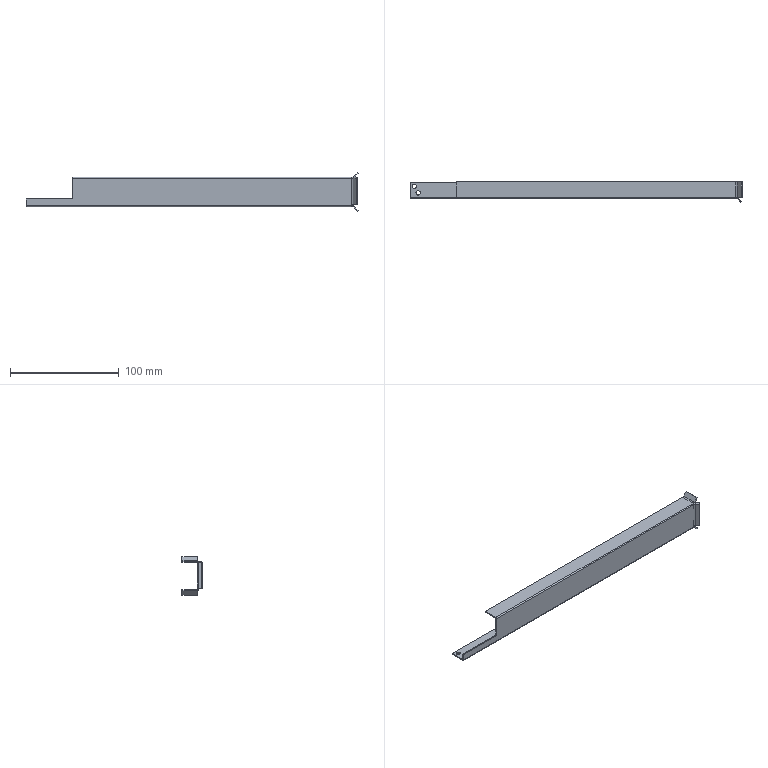Part | NX | 1 solid | 39 faces | box 305.707 x 18.464 x 35.21 mm | volume 15234 mm3 | plane 24 | cylinder 14 | torus 1 | commonest cylinder face diameters 4 x6 6 x4 2 x3 2.56 x1
STEP:
#1=CARTESIAN_POINT('',(150.133,7.5,151.5));
#2=VERTEX_POINT('',#1);
#3=CARTESIAN_POINT('',(150.133,-6.501,151.5));
#4=VERTEX_POINT('',#3);
#5=CARTESIAN_POINT('',(150.133,7.5,151.5));
#6=DIRECTION('',(0.,-1.,0.));
#7=VECTOR('',#6,1000.);
#8=LINE('',#5,#7);
#9=EDGE_CURVE('',#2,#4,#8,.T.);
#10=ORIENTED_EDGE('',*,*,#9,.F.);
#11=CARTESIAN_POINT('',(-107.,7.5,151.5));
#12=VERTEX_POINT('',#11);
#13=CARTESIAN_POINT('',(-107.,7.5,151.5));
#14=DIRECTION('',(1.,0.,0.));
#15=VECTOR('',#14,1000.);
#16=LINE('',#13,#15);
#17=EDGE_CURVE('',#12,#2,#16,.T.);
#18=ORIENTED_EDGE('',*,*,#17,.F.);
#19=CARTESIAN_POINT('',(-107.,-6.5,151.5));
#20=VERTEX_POINT('',#19);
#21=CARTESIAN_POINT('',(-107.,7.5,151.5));
#22=DIRECTION('',(0.,-1.,0.));
#23=VECTOR('',#22,1000.);
#24=LINE('',#21,#23);
#25=EDGE_CURVE('',#12,#20,#24,.T.);
#26=ORIENTED_EDGE('',*,*,#25,.T.);
#27=CARTESIAN_POINT('',(150.,-6.5,151.5));
#28=VERTEX_POINT('',#27);
#29=CARTESIAN_POINT('',(150.722,-6.5,151.5));
#30=DIRECTION('',(1.,0.,0.));
#31=VECTOR('',#30,1000.);
#32=LINE('',#29,#31);
#33=EDGE_CURVE('',#20,#28,#32,.T.);
#34=ORIENTED_EDGE('',*,*,#33,.T.);
#35=CARTESIAN_POINT('',(150.,-9.5,151.5));
#36=DIRECTION('',(0.,0.,1.));
#37=DIRECTION('',(0.04435,0.999,0.));
#38=AXIS2_PLACEMENT_3D('',#35,#36,#37);
#39=CIRCLE('',#38,3.);
#40=EDGE_CURVE('',#4,#28,#39,.T.);
#41=ORIENTED_EDGE('',*,*,#40,.F.);
#42=EDGE_LOOP('',(#10,#18,#26,#34,#41));
#43=FACE_BOUND('',#42,.T.);
#44=CARTESIAN_POINT('',(0.,0.,151.5));
#45=DIRECTION('',(0.,0.,1.));
#46=DIRECTION('',(1.,0.,0.));
#47=AXIS2_PLACEMENT_3D('',#44,#45,#46);
#48=PLANE('',#47);
#49=ADVANCED_FACE('',(#43),#48,.T.);
#50=CARTESIAN_POINT('',(151.547,7.5,152.086));
#51=VERTEX_POINT('',#50);
#52=CARTESIAN_POINT('',(150.133,7.5,153.5));
#53=DIRECTION('',(0.,1.,0.));
#54=DIRECTION('',(0.7071,0.,-0.7071));
#55=AXIS2_PLACEMENT_3D('',#52,#53,#54);
#56=CIRCLE('',#55,2.);
#57=EDGE_CURVE('',#51,#2,#56,.T.);
#58=ORIENTED_EDGE('',*,*,#57,.T.);
#59=ORIENTED_EDGE('',*,*,#9,.T.);
#60=CARTESIAN_POINT('',(151.547,-6.5,152.086));
#61=VERTEX_POINT('',#60);
#62=CARTESIAN_POINT('',(150.133,-6.5,153.5));
#63=DIRECTION('',(0.,-1.,0.));
#64=DIRECTION('',(0.,0.,-1.));
#65=AXIS2_PLACEMENT_3D('',#62,#63,#64);
#66=CIRCLE('',#65,2.);
#67=EDGE_CURVE('',#4,#61,#66,.T.);
#68=ORIENTED_EDGE('',*,*,#67,.T.);
#69=CARTESIAN_POINT('',(151.547,7.5,152.086));
#70=DIRECTION('',(0.,-1.,0.));
#71=VECTOR('',#70,1000.);
#72=LINE('',#69,#71);
#73=EDGE_CURVE('',#51,#61,#72,.T.);
#74=ORIENTED_EDGE('',*,*,#73,.F.);
#75=EDGE_LOOP('',(#58,#59,#68,#74));
#76=FACE_BOUND('',#75,.T.);
#77=CARTESIAN_POINT('',(150.133,7.5,153.5));
#78=DIRECTION('',(0.,-1.,0.));
#79=DIRECTION('',(0.,0.,-1.));
#80=AXIS2_PLACEMENT_3D('',#77,#78,#79);
#81=CYLINDRICAL_SURFACE('',#80,2.);
#82=ADVANCED_FACE('',(#76),#81,.F.);
#83=ORIENTED_EDGE('',*,*,#17,.T.);
#84=ORIENTED_EDGE('',*,*,#57,.F.);
#85=CARTESIAN_POINT('',(155.,7.5,155.539));
#86=VERTEX_POINT('',#85);
#87=CARTESIAN_POINT('',(155.,7.5,155.539));
#88=DIRECTION('',(-0.7071,0.,-0.7071));
#89=VECTOR('',#88,1000.);
#90=LINE('',#87,#89);
#91=EDGE_CURVE('',#86,#51,#90,.T.);
#92=ORIENTED_EDGE('',*,*,#91,.F.);
#93=CARTESIAN_POINT('',(155.707,7.5,154.831));
#94=VERTEX_POINT('',#93);
#95=CARTESIAN_POINT('',(155.707,7.5,154.831));
#96=DIRECTION('',(-0.7071,0.,0.7071));
#97=VECTOR('',#96,1000.);
#98=LINE('',#95,#97);
#99=EDGE_CURVE('',#94,#86,#98,.T.);
#100=ORIENTED_EDGE('',*,*,#99,.F.);
#101=CARTESIAN_POINT('',(152.254,7.5,151.378));
#102=VERTEX_POINT('',#101);
#103=CARTESIAN_POINT('',(152.254,7.5,151.378));
#104=DIRECTION('',(0.7071,0.,0.7071));
#105=VECTOR('',#104,1000.);
#106=LINE('',#103,#105);
#107=EDGE_CURVE('',#102,#94,#106,.T.);
#108=ORIENTED_EDGE('',*,*,#107,.F.);
#109=CARTESIAN_POINT('',(150.133,7.5,150.5));
#110=VERTEX_POINT('',#109);
#111=CARTESIAN_POINT('',(150.133,7.5,153.5));
#112=DIRECTION('',(0.,-1.,0.));
#113=DIRECTION('',(0.00000176,0.,-1.));
#114=AXIS2_PLACEMENT_3D('',#111,#112,#113);
#115=CIRCLE('',#114,3.);
#116=EDGE_CURVE('',#110,#102,#115,.T.);
#117=ORIENTED_EDGE('',*,*,#116,.F.);
#118=CARTESIAN_POINT('',(149.991,7.5,150.502));
#119=VERTEX_POINT('',#118);
#120=CARTESIAN_POINT('',(150.133,7.5,153.5));
#121=DIRECTION('',(0.,-1.,0.));
#122=DIRECTION('',(0.00000176,0.,-1.));
#123=AXIS2_PLACEMENT_3D('',#120,#121,#122);
#124=CIRCLE('',#123,3.);
#125=EDGE_CURVE('',#119,#110,#124,.T.);
#126=ORIENTED_EDGE('',*,*,#125,.F.);
#127=CARTESIAN_POINT('',(-107.,7.5,150.5));
#128=VERTEX_POINT('',#127);
#129=CARTESIAN_POINT('',(149.991,7.5,150.501));
#130=CARTESIAN_POINT('',(64.328,7.5,150.501));
#131=CARTESIAN_POINT('',(-21.336,7.5,150.501));
#132=CARTESIAN_POINT('',(-107.,7.5,150.5));
#133=B_SPLINE_CURVE_WITH_KNOTS('',3,(#129,#130,#131,#132),.UNSPECIFIED.,.F.,.F.,(4,4),(0.,1.),.UNSPECIFIED.);
#134=EDGE_CURVE('',#119,#128,#133,.T.);
#135=ORIENTED_EDGE('',*,*,#134,.T.);
#136=CARTESIAN_POINT('',(-107.,7.5,150.5));
#137=DIRECTION('',(0.,0.,1.));
#138=VECTOR('',#137,1000.);
#139=LINE('',#136,#138);
#140=EDGE_CURVE('',#128,#12,#139,.T.);
#141=ORIENTED_EDGE('',*,*,#140,.T.);
#142=EDGE_LOOP('',(#83,#84,#92,#100,#108,#117,#126,#135,#141));
#143=FACE_BOUND('',#142,.T.);
#144=CARTESIAN_POINT('',(0.,7.5,151.5));
#145=DIRECTION('',(0.,-1.,0.));
#146=DIRECTION('',(0.,0.,-1.));
#147=AXIS2_PLACEMENT_3D('',#144,#145,#146);
#148=PLANE('',#147);
#149=ADVANCED_FACE('',(#143),#148,.F.);
#150=CARTESIAN_POINT('',(-107.,-7.5,150.5));
#151=VERTEX_POINT('',#150);
#152=CARTESIAN_POINT('',(-107.,-6.5,150.5));
#153=DIRECTION('',(1.,0.,0.));
#154=DIRECTION('',(0.,0.,1.));
#155=AXIS2_PLACEMENT_3D('',#152,#153,#154);
#156=CIRCLE('',#155,1.);
#157=EDGE_CURVE('',#20,#151,#156,.T.);
#158=ORIENTED_EDGE('',*,*,#157,.F.);
#159=ORIENTED_EDGE('',*,*,#25,.F.);
#160=ORIENTED_EDGE('',*,*,#140,.F.);
#161=CARTESIAN_POINT('',(-107.,-6.5,150.5));
#162=VERTEX_POINT('',#161);
#163=CARTESIAN_POINT('',(-107.,7.5,150.5));
#164=CARTESIAN_POINT('',(-107.,2.833,150.5));
#165=CARTESIAN_POINT('',(-107.,-1.833,150.5));
#166=CARTESIAN_POINT('',(-107.,-6.5,150.5));
#167=B_SPLINE_CURVE_WITH_KNOTS('',3,(#163,#164,#165,#166),.UNSPECIFIED.,.F.,.F.,(4,4),(0.,1.),.UNSPECIFIED.);
#168=EDGE_CURVE('',#128,#162,#167,.T.);
#169=ORIENTED_EDGE('',*,*,#168,.T.);
#170=CARTESIAN_POINT('',(-107.,-6.5,131.5));
#171=VERTEX_POINT('',#170);
#172=CARTESIAN_POINT('',(-107.,-6.5,131.5));
#173=DIRECTION('',(0.,0.,1.));
#174=VECTOR('',#173,1000.);
#175=LINE('',#172,#174);
#176=EDGE_CURVE('',#171,#162,#175,.T.);
#177=ORIENTED_EDGE('',*,*,#176,.F.);
#178=CARTESIAN_POINT('',(-107.,-7.5,131.5));
#179=VERTEX_POINT('',#178);
#180=CARTESIAN_POINT('',(-107.,-6.5,131.5));
#181=DIRECTION('',(0.,-1.,0.));
#182=VECTOR('',#181,1000.);
#183=LINE('',#180,#182);
#184=EDGE_CURVE('',#171,#179,#183,.T.);
#185=ORIENTED_EDGE('',*,*,#184,.T.);
#186=CARTESIAN_POINT('',(-107.,-7.5,131.5));
#187=DIRECTION('',(0.,0.,1.));
#188=VECTOR('',#187,1000.);
#189=LINE('',#186,#188);
#190=EDGE_CURVE('',#179,#151,#189,.T.);
#191=ORIENTED_EDGE('',*,*,#190,.T.);
#192=EDGE_LOOP('',(#158,#159,#160,#169,#177,#185,#191));
#193=FACE_BOUND('',#192,.T.);
#194=CARTESIAN_POINT('',(-107.,-7.5,151.5));
#195=DIRECTION('',(-1.,0.,0.));
#196=DIRECTION('',(0.,0.,1.));
#197=AXIS2_PLACEMENT_3D('',#194,#195,#196);
#198=PLANE('',#197);
#199=ADVANCED_FACE('',(#193),#198,.T.);
#200=CARTESIAN_POINT('',(150.,-7.5,150.5));
#201=VERTEX_POINT('',#200);
#202=CARTESIAN_POINT('',(150.,-7.5,150.5));
#203=DIRECTION('',(-1.,0.,0.));
#204=VECTOR('',#203,1000.);
#205=LINE('',#202,#204);
#206=EDGE_CURVE('',#201,#151,#205,.T.);
#207=ORIENTED_EDGE('',*,*,#206,.F.);
#208=CARTESIAN_POINT('',(150.,-6.5,150.5));
#209=DIRECTION('',(-1.,0.,0.));
#210=DIRECTION('',(0.,-1.,0.));
#211=AXIS2_PLACEMENT_3D('',#208,#209,#210);
#212=CIRCLE('',#211,1.);
#213=EDGE_CURVE('',#201,#28,#212,.T.);
#214=ORIENTED_EDGE('',*,*,#213,.T.);
#215=ORIENTED_EDGE('',*,*,#33,.F.);
#216=ORIENTED_EDGE('',*,*,#157,.T.);
#217=EDGE_LOOP('',(#207,#214,#215,#216));
#218=FACE_BOUND('',#217,.T.);
#219=CARTESIAN_POINT('',(150.722,-6.5,150.5));
#220=DIRECTION('',(1.,0.,0.));
#221=DIRECTION('',(0.,0.,1.));
#222=AXIS2_PLACEMENT_3D('',#219,#220,#221);
#223=CYLINDRICAL_SURFACE('',#222,1.);
#224=ADVANCED_FACE('',(#218),#223,.T.);
#225=ORIENTED_EDGE('',*,*,#206,.T.);
#226=ORIENTED_EDGE('',*,*,#190,.F.);
#227=CARTESIAN_POINT('',(-150.,-7.5,131.5));
#228=VERTEX_POINT('',#227);
#229=CARTESIAN_POINT('',(-107.,-7.5,131.5));
#230=DIRECTION('',(-1.,0.,0.));
#231=VECTOR('',#230,1000.);
#232=LINE('',#229,#231);
#233=EDGE_CURVE('',#179,#228,#232,.T.);
#234=ORIENTED_EDGE('',*,*,#233,.T.);
#235=CARTESIAN_POINT('',(-150.,-7.5,125.5));
#236=VERTEX_POINT('',#235);
#237=CARTESIAN_POINT('',(-150.,-7.5,125.5));
#238=DIRECTION('',(0.,0.,1.));
#239=VECTOR('',#238,1000.);
#240=LINE('',#237,#239);
#241=EDGE_CURVE('',#236,#228,#240,.T.);
#242=ORIENTED_EDGE('',*,*,#241,.F.);
#243=CARTESIAN_POINT('',(150.,-7.5,125.5));
#244=VERTEX_POINT('',#243);
#245=CARTESIAN_POINT('',(-150.,-7.5,125.5));
#246=DIRECTION('',(1.,0.,0.));
#247=VECTOR('',#246,1000.);
#248=LINE('',#245,#247);
#249=EDGE_CURVE('',#236,#244,#248,.T.);
#250=ORIENTED_EDGE('',*,*,#249,.T.);
#251=CARTESIAN_POINT('',(150.,-7.5,126.5));
#252=VERTEX_POINT('',#251);
#253=CARTESIAN_POINT('',(150.,-7.5,125.5));
#254=DIRECTION('',(0.,0.,1.));
#255=VECTOR('',#254,1000.);
#256=LINE('',#253,#255);
#257=EDGE_CURVE('',#244,#252,#256,.T.);
#258=ORIENTED_EDGE('',*,*,#257,.T.);
#259=CARTESIAN_POINT('',(150.,-7.5,151.5));
#260=DIRECTION('',(0.,0.,1.));
#261=VECTOR('',#260,1000.);
#262=LINE('',#259,#261);
#263=EDGE_CURVE('',#252,#201,#262,.T.);
#264=ORIENTED_EDGE('',*,*,#263,.T.);
#265=EDGE_LOOP('',(#225,#226,#234,#242,#250,#258,#264));
#266=FACE_BOUND('',#265,.T.);
#267=CARTESIAN_POINT('',(-150.,-7.5,151.5));
#268=DIRECTION('',(0.,1.,0.));
#269=DIRECTION('',(1.,0.,0.));
#270=AXIS2_PLACEMENT_3D('',#267,#268,#269);
#271=PLANE('',#270);
#272=ADVANCED_FACE('',(#266),#271,.F.);
#273=CARTESIAN_POINT('',(151.414,-8.086,150.5));
#274=VERTEX_POINT('',#273);
#275=CARTESIAN_POINT('',(150.,-9.5,150.5));
#276=DIRECTION('',(0.,0.,1.));
#277=DIRECTION('',(1.,0.,0.));
#278=AXIS2_PLACEMENT_3D('',#275,#276,#277);
#279=CIRCLE('',#278,2.);
#280=EDGE_CURVE('',#274,#201,#279,.T.);
#281=ORIENTED_EDGE('',*,*,#280,.T.);
#282=ORIENTED_EDGE('',*,*,#263,.F.);
#283=CARTESIAN_POINT('',(151.414,-8.086,126.5));
#284=VERTEX_POINT('',#283);
#285=CARTESIAN_POINT('',(150.,-9.5,126.5));
#286=DIRECTION('',(0.,0.,-1.));
#287=DIRECTION('',(0.,1.,0.));
#288=AXIS2_PLACEMENT_3D('',#285,#286,#287);
#289=CIRCLE('',#288,2.);
#290=EDGE_CURVE('',#252,#284,#289,.T.);
#291=ORIENTED_EDGE('',*,*,#290,.T.);
#292=CARTESIAN_POINT('',(151.414,-8.086,150.5));
#293=DIRECTION('',(0.,0.,-1.));
#294=VECTOR('',#293,1000.);
#295=LINE('',#292,#294);
#296=EDGE_CURVE('',#274,#284,#295,.T.);
#297=ORIENTED_EDGE('',*,*,#296,.F.);
#298=EDGE_LOOP('',(#281,#282,#291,#297));
#299=FACE_BOUND('',#298,.T.);
#300=CARTESIAN_POINT('',(150.,-9.5,151.5));
#301=DIRECTION('',(0.,0.,1.));
#302=DIRECTION('',(0.,1.,0.));
#303=AXIS2_PLACEMENT_3D('',#300,#301,#302);
#304=CYLINDRICAL_SURFACE('',#303,2.);
#305=ADVANCED_FACE('',(#299),#304,.F.);
#306=CARTESIAN_POINT('',(152.121,-7.379,151.5));
#307=VERTEX_POINT('',#306);
#308=CARTESIAN_POINT('',(150.,-9.5,151.5));
#309=DIRECTION('',(0.,0.,-1.));
#310=DIRECTION('',(0.04432,0.999,0.));
#311=AXIS2_PLACEMENT_3D('',#308,#309,#310);
#312=CIRCLE('',#311,3.);
#313=EDGE_CURVE('',#4,#307,#312,.T.);
#314=ORIENTED_EDGE('',*,*,#313,.F.);
#315=ORIENTED_EDGE('',*,*,#40,.T.);
#316=ORIENTED_EDGE('',*,*,#213,.F.);
#317=ORIENTED_EDGE('',*,*,#280,.F.);
#318=CARTESIAN_POINT('',(152.121,-7.379,150.5));
#319=DIRECTION('',(0.7071,-0.7071,0.));
#320=DIRECTION('',(0.,0.,1.));
#321=AXIS2_PLACEMENT_3D('',#318,#319,#320);
#322=CIRCLE('',#321,1.);
#323=EDGE_CURVE('',#307,#274,#322,.T.);
#324=ORIENTED_EDGE('',*,*,#323,.F.);
#325=EDGE_LOOP('',(#314,#315,#316,#317,#324));
#326=FACE_BOUND('',#325,.T.);
#327=CARTESIAN_POINT('',(150.,-9.5,150.5));
#328=DIRECTION('',(0.,0.,1.));
#329=DIRECTION('',(1.,0.,0.));
#330=AXIS2_PLACEMENT_3D('',#327,#328,#329);
#331=TOROIDAL_SURFACE('',#330,3.,1.);
#332=ADVANCED_FACE('',(#326),#331,.T.);
#333=CARTESIAN_POINT('',(152.121,-7.379,126.5));
#334=VERTEX_POINT('',#333);
#335=CARTESIAN_POINT('',(152.121,-7.379,126.5));
#336=DIRECTION('',(0.,0.,1.));
#337=VECTOR('',#336,1000.);
#338=LINE('',#335,#337);
#339=EDGE_CURVE('',#334,#307,#338,.T.);
#340=ORIENTED_EDGE('',*,*,#339,.F.);
#341=CARTESIAN_POINT('',(150.,-6.5,126.5));
#342=VERTEX_POINT('',#341);
#343=CARTESIAN_POINT('',(150.,-9.5,126.5));
#344=DIRECTION('',(0.,0.,1.));
#345=DIRECTION('',(0.7071,0.7071,0.));
#346=AXIS2_PLACEMENT_3D('',#343,#344,#345);
#347=CIRCLE('',#346,3.);
#348=EDGE_CURVE('',#334,#342,#347,.T.);
#349=ORIENTED_EDGE('',*,*,#348,.T.);
#350=CARTESIAN_POINT('',(150.,-6.5,150.502));
#351=VERTEX_POINT('',#350);
#352=CARTESIAN_POINT('',(150.,-6.5,151.5));
#353=DIRECTION('',(0.,0.,1.));
#354=VECTOR('',#353,1000.);
#355=LINE('',#352,#354);
#356=EDGE_CURVE('',#342,#351,#355,.T.);
#357=ORIENTED_EDGE('',*,*,#356,.T.);
#358=CARTESIAN_POINT('',(150.,-6.5,151.5));
#359=VERTEX_POINT('',#358);
#360=CARTESIAN_POINT('',(150.,-6.5,151.5));
#361=DIRECTION('',(0.,0.,1.));
#362=VECTOR('',#361,1000.);
#363=LINE('',#360,#362);
#364=EDGE_CURVE('',#351,#359,#363,.T.);
#365=ORIENTED_EDGE('',*,*,#364,.T.);
#366=CARTESIAN_POINT('',(150.133,-6.5,151.5));
#367=CARTESIAN_POINT('',(150.089,-6.5,151.5));
#368=CARTESIAN_POINT('',(150.044,-6.5,151.5));
#369=CARTESIAN_POINT('',(150.,-6.5,151.5));
#370=B_SPLINE_CURVE_WITH_KNOTS('',3,(#366,#367,#368,#369),.UNSPECIFIED.,.F.,.F.,(4,4),(0.,1.),.UNSPECIFIED.);
#371=EDGE_CURVE('',#4,#359,#370,.T.);
#372=ORIENTED_EDGE('',*,*,#371,.F.);
#373=ORIENTED_EDGE('',*,*,#313,.T.);
#374=EDGE_LOOP('',(#340,#349,#357,#365,#372,#373));
#375=FACE_BOUND('',#374,.T.);
#376=CARTESIAN_POINT('',(150.,-9.5,151.5));
#377=DIRECTION('',(0.,0.,1.));
#378=DIRECTION('',(0.,1.,0.));
#379=AXIS2_PLACEMENT_3D('',#376,#377,#378);
#380=CYLINDRICAL_SURFACE('',#379,3.);
#381=ADVANCED_FACE('',(#375),#380,.T.);
#382=CARTESIAN_POINT('',(155.,-10.257,151.5));
#383=VERTEX_POINT('',#382);
#384=CARTESIAN_POINT('',(155.489,-10.746,151.5));
#385=DIRECTION('',(0.7071,-0.7071,0.));
#386=VECTOR('',#385,1000.);
#387=LINE('',#384,#386);
#388=EDGE_CURVE('',#307,#383,#387,.T.);
#389=ORIENTED_EDGE('',*,*,#388,.T.);
#390=CARTESIAN_POINT('',(155.,-10.257,126.5));
#391=VERTEX_POINT('',#390);
#392=CARTESIAN_POINT('',(155.,-10.257,126.5));
#393=DIRECTION('',(0.,0.,1.));
#394=VECTOR('',#393,1000.);
#395=LINE('',#392,#394);
#396=EDGE_CURVE('',#391,#383,#395,.T.);
#397=ORIENTED_EDGE('',*,*,#396,.F.);
#398=CARTESIAN_POINT('',(155.,-10.257,126.5));
#399=DIRECTION('',(-0.7071,0.7071,0.));
#400=VECTOR('',#399,1000.);
#401=LINE('',#398,#400);
#402=EDGE_CURVE('',#391,#334,#401,.T.);
#403=ORIENTED_EDGE('',*,*,#402,.T.);
#404=ORIENTED_EDGE('',*,*,#339,.T.);
#405=EDGE_LOOP('',(#389,#397,#403,#404));
#406=FACE_BOUND('',#405,.T.);
#407=CARTESIAN_POINT('',(155.,-10.257,151.5));
#408=DIRECTION('',(-0.7071,-0.7071,0.));
#409=DIRECTION('',(-0.7071,0.7071,0.));
#410=AXIS2_PLACEMENT_3D('',#407,#408,#409);
#411=PLANE('',#410);
#412=ADVANCED_FACE('',(#406),#411,.F.);
#413=CARTESIAN_POINT('',(154.293,-10.964,150.5));
#414=VERTEX_POINT('',#413);
#415=CARTESIAN_POINT('',(154.293,-10.964,150.5));
#416=DIRECTION('',(-0.7071,0.7071,0.));
#417=VECTOR('',#416,1000.);
#418=LINE('',#415,#417);
#419=EDGE_CURVE('',#414,#274,#418,.T.);
#420=ORIENTED_EDGE('',*,*,#419,.F.);
#421=CARTESIAN_POINT('',(155.,-10.257,150.5));
#422=DIRECTION('',(-0.7071,0.7071,0.));
#423=DIRECTION('',(-0.7071,-0.7071,0.));
#424=AXIS2_PLACEMENT_3D('',#421,#422,#423);
#425=CIRCLE('',#424,1.);
#426=EDGE_CURVE('',#414,#383,#425,.T.);
#427=ORIENTED_EDGE('',*,*,#426,.T.);
#428=ORIENTED_EDGE('',*,*,#388,.F.);
#429=ORIENTED_EDGE('',*,*,#323,.T.);
#430=EDGE_LOOP('',(#420,#427,#428,#429));
#431=FACE_BOUND('',#430,.T.);
#432=CARTESIAN_POINT('',(155.489,-10.746,150.5));
#433=DIRECTION('',(0.7071,-0.7071,0.));
#434=DIRECTION('',(0.,0.,1.));
#435=AXIS2_PLACEMENT_3D('',#432,#433,#434);
#436=CYLINDRICAL_SURFACE('',#435,1.);
#437=ADVANCED_FACE('',(#431),#436,.T.);
#438=ORIENTED_EDGE('',*,*,#419,.T.);
#439=ORIENTED_EDGE('',*,*,#296,.T.);
#440=CARTESIAN_POINT('',(154.293,-10.964,126.5));
#441=VERTEX_POINT('',#440);
#442=CARTESIAN_POINT('',(151.414,-8.086,126.5));
#443=DIRECTION('',(0.7071,-0.7071,0.));
#444=VECTOR('',#443,1000.);
#445=LINE('',#442,#444);
#446=EDGE_CURVE('',#284,#441,#445,.T.);
#447=ORIENTED_EDGE('',*,*,#446,.T.);
#448=CARTESIAN_POINT('',(154.293,-10.964,126.5));
#449=DIRECTION('',(0.,0.,1.));
#450=VECTOR('',#449,1000.);
#451=LINE('',#448,#450);
#452=EDGE_CURVE('',#441,#414,#451,.T.);
#453=ORIENTED_EDGE('',*,*,#452,.T.);
#454=EDGE_LOOP('',(#438,#439,#447,#453));
#455=FACE_BOUND('',#454,.T.);
#456=CARTESIAN_POINT('',(151.414,-8.086,151.5));
#457=DIRECTION('',(0.7071,0.7071,0.));
#458=DIRECTION('',(0.,0.,-1.));
#459=AXIS2_PLACEMENT_3D('',#456,#457,#458);
#460=PLANE('',#459);
#461=ADVANCED_FACE('',(#455),#460,.F.);
#462=ORIENTED_EDGE('',*,*,#426,.F.);
#463=ORIENTED_EDGE('',*,*,#452,.F.);
#464=CARTESIAN_POINT('',(154.293,-10.964,126.5));
#465=DIRECTION('',(0.7071,0.7071,0.));
#466=VECTOR('',#465,1000.);
#467=LINE('',#464,#466);
#468=EDGE_CURVE('',#441,#391,#467,.T.);
#469=ORIENTED_EDGE('',*,*,#468,.T.);
#470=ORIENTED_EDGE('',*,*,#396,.T.);
#471=EDGE_LOOP('',(#462,#463,#469,#470));
#472=FACE_BOUND('',#471,.T.);
#473=CARTESIAN_POINT('',(154.293,-10.964,151.5));
#474=DIRECTION('',(-0.7071,0.7071,0.));
#475=DIRECTION('',(0.,0.,1.));
#476=AXIS2_PLACEMENT_3D('',#473,#474,#475);
#477=PLANE('',#476);
#478=ADVANCED_FACE('',(#472),#477,.F.);
#479=CARTESIAN_POINT('',(150.,-6.5,126.5));
#480=DIRECTION('',(-0.000001634,-1.,0.));
#481=VECTOR('',#480,1000.);
#482=LINE('',#479,#481);
#483=EDGE_CURVE('',#342,#252,#482,.T.);
#484=ORIENTED_EDGE('',*,*,#483,.F.);
#485=ORIENTED_EDGE('',*,*,#348,.F.);
#486=ORIENTED_EDGE('',*,*,#402,.F.);
#487=ORIENTED_EDGE('',*,*,#468,.F.);
#488=ORIENTED_EDGE('',*,*,#446,.F.);
#489=ORIENTED_EDGE('',*,*,#290,.F.);
#490=EDGE_LOOP('',(#484,#485,#486,#487,#488,#489));
#491=FACE_BOUND('',#490,.T.);
#492=CARTESIAN_POINT('',(0.,0.,126.5));
#493=DIRECTION('',(0.,0.,1.));
#494=DIRECTION('',(1.,0.,0.));
#495=AXIS2_PLACEMENT_3D('',#492,#493,#494);
#496=PLANE('',#495);
#497=ADVANCED_FACE('',(#491),#496,.F.);
#498=CARTESIAN_POINT('',(150.,-6.5,124.5));
#499=VERTEX_POINT('',#498);
#500=CARTESIAN_POINT('',(150.,-6.5,125.5));
#501=DIRECTION('',(-1.,0.,0.));
#502=DIRECTION('',(0.,0.,-1.));
#503=AXIS2_PLACEMENT_3D('',#500,#501,#502);
#504=CIRCLE('',#503,1.);
#505=EDGE_CURVE('',#499,#244,#504,.T.);
#506=ORIENTED_EDGE('',*,*,#505,.F.);
#507=CARTESIAN_POINT('',(150.,-6.5,125.5));
#508=VERTEX_POINT('',#507);
#509=CARTESIAN_POINT('',(150.,-6.5,125.5));
#510=DIRECTION('',(0.,0.,-1.));
#511=VECTOR('',#510,1000.);
#512=LINE('',#509,#511);
#513=EDGE_CURVE('',#508,#499,#512,.T.);
#514=ORIENTED_EDGE('',*,*,#513,.F.);
#515=CARTESIAN_POINT('',(150.,-6.5,125.5));
#516=DIRECTION('',(0.000001634,0.,1.));
#517=VECTOR('',#516,1000.);
#518=LINE('',#515,#517);
#519=EDGE_CURVE('',#508,#342,#518,.T.);
#520=ORIENTED_EDGE('',*,*,#519,.T.);
#521=ORIENTED_EDGE('',*,*,#483,.T.);
#522=ORIENTED_EDGE('',*,*,#257,.F.);
#523=EDGE_LOOP('',(#506,#514,#520,#521,#522));
#524=FACE_BOUND('',#523,.T.);
#525=CARTESIAN_POINT('',(150.,-7.5,151.5));
#526=DIRECTION('',(-1.,0.,0.));
#527=DIRECTION('',(0.,0.,1.));
#528=AXIS2_PLACEMENT_3D('',#525,#526,#527);
#529=PLANE('',#528);
#530=ADVANCED_FACE('',(#524),#529,.F.);
#531=CARTESIAN_POINT('',(-150.,-6.5,124.5));
#532=VERTEX_POINT('',#531);
#533=CARTESIAN_POINT('',(-150.508,-6.5,124.5));
#534=DIRECTION('',(-1.,0.,0.));
#535=VECTOR('',#534,1000.);
#536=LINE('',#533,#535);
#537=EDGE_CURVE('',#499,#532,#536,.T.);
#538=ORIENTED_EDGE('',*,*,#537,.F.);
#539=ORIENTED_EDGE('',*,*,#505,.T.);
#540=ORIENTED_EDGE('',*,*,#249,.F.);
#541=CARTESIAN_POINT('',(-150.,-6.5,125.5));
#542=DIRECTION('',(1.,0.,0.));
#543=DIRECTION('',(0.,-1.,0.));
#544=AXIS2_PLACEMENT_3D('',#541,#542,#543);
#545=CIRCLE('',#544,1.);
#546=EDGE_CURVE('',#236,#532,#545,.T.);
#547=ORIENTED_EDGE('',*,*,#546,.T.);
#548=EDGE_LOOP('',(#538,#539,#540,#547));
#549=FACE_BOUND('',#548,.T.);
#550=CARTESIAN_POINT('',(-150.508,-6.5,125.5));
#551=DIRECTION('',(-1.,0.,0.));
#552=DIRECTION('',(0.,0.,-1.));
#553=AXIS2_PLACEMENT_3D('',#550,#551,#552);
#554=CYLINDRICAL_SURFACE('',#553,1.);
#555=ADVANCED_FACE('',(#549),#554,.T.);
#556=ORIENTED_EDGE('',*,*,#537,.T.);
#557=CARTESIAN_POINT('',(-150.,7.5,124.5));
#558=VERTEX_POINT('',#557);
#559=CARTESIAN_POINT('',(-150.,-6.5,124.5));
#560=DIRECTION('',(0.,1.,0.));
#561=VECTOR('',#560,1000.);
#562=LINE('',#559,#561);
#563=EDGE_CURVE('',#532,#558,#562,.T.);
#564=ORIENTED_EDGE('',*,*,#563,.T.);
#565=CARTESIAN_POINT('',(150.298,7.5,124.5));
#566=VERTEX_POINT('',#565);
#567=CARTESIAN_POINT('',(150.298,7.5,124.5));
#568=DIRECTION('',(-1.,0.,0.));
#569=VECTOR('',#568,1000.);
#570=LINE('',#567,#569);
#571=EDGE_CURVE('',#566,#558,#570,.T.);
#572=ORIENTED_EDGE('',*,*,#571,.F.);
#573=CARTESIAN_POINT('',(150.298,-6.5,124.5));
#574=VERTEX_POINT('',#573);
#575=CARTESIAN_POINT('',(150.298,7.5,124.5));
#576=DIRECTION('',(0.,1.,0.));
#577=VECTOR('',#576,1000.);
#578=LINE('',#575,#577);
#579=EDGE_CURVE('',#574,#566,#578,.T.);
#580=ORIENTED_EDGE('',*,*,#579,.F.);
#581=CARTESIAN_POINT('',(150.,-6.5,124.5));
#582=DIRECTION('',(1.,0.,0.));
#583=VECTOR('',#582,1000.);
#584=LINE('',#581,#583);
#585=EDGE_CURVE('',#499,#574,#584,.T.);
#586=ORIENTED_EDGE('',*,*,#585,.F.);
#587=EDGE_LOOP('',(#556,#564,#572,#580,#586));
#588=FACE_BOUND('',#587,.T.);
#589=CARTESIAN_POINT('',(-144.,3.5,124.5));
#590=VERTEX_POINT('',#589);
#591=CARTESIAN_POINT('',(-148.,3.5,124.5));
#592=VERTEX_POINT('',#591);
#593=CARTESIAN_POINT('',(-146.,3.5,124.5));
#594=DIRECTION('',(0.,0.,-1.));
#595=DIRECTION('',(-1.,0.,0.));
#596=AXIS2_PLACEMENT_3D('',#593,#594,#595);
#597=CIRCLE('',#596,2.);
#598=EDGE_CURVE('',#590,#592,#597,.T.);
#599=ORIENTED_EDGE('',*,*,#598,.F.);
#600=CARTESIAN_POINT('',(-146.,3.5,124.5));
#601=DIRECTION('',(0.,0.,-1.));
#602=DIRECTION('',(-1.,0.,0.));
#603=AXIS2_PLACEMENT_3D('',#600,#601,#602);
#604=CIRCLE('',#603,2.);
#605=EDGE_CURVE('',#592,#590,#604,.T.);
#606=ORIENTED_EDGE('',*,*,#605,.F.);
#607=EDGE_LOOP('',(#599,#606));
#608=FACE_BOUND('',#607,.T.);
#609=CARTESIAN_POINT('',(-140.5,-2.562,124.5));
#610=VERTEX_POINT('',#609);
#611=CARTESIAN_POINT('',(-144.5,-2.562,124.5));
#612=VERTEX_POINT('',#611);
#613=CARTESIAN_POINT('',(-142.5,-2.562,124.5));
#614=DIRECTION('',(0.,0.,-1.));
#615=DIRECTION('',(-1.,0.,0.));
#616=AXIS2_PLACEMENT_3D('',#613,#614,#615);
#617=CIRCLE('',#616,2.);
#618=EDGE_CURVE('',#610,#612,#617,.T.);
#619=ORIENTED_EDGE('',*,*,#618,.F.);
#620=CARTESIAN_POINT('',(-142.5,-2.562,124.5));
#621=DIRECTION('',(0.,0.,-1.));
#622=DIRECTION('',(-1.,0.,0.));
#623=AXIS2_PLACEMENT_3D('',#620,#621,#622);
#624=CIRCLE('',#623,2.);
#625=EDGE_CURVE('',#612,#610,#624,.T.);
#626=ORIENTED_EDGE('',*,*,#625,.F.);
#627=EDGE_LOOP('',(#619,#626));
#628=FACE_BOUND('',#627,.T.);
#629=CARTESIAN_POINT('',(0.,0.,124.5));
#630=DIRECTION('',(0.,0.,1.));
#631=DIRECTION('',(1.,0.,0.));
#632=AXIS2_PLACEMENT_3D('',#629,#630,#631);
#633=PLANE('',#632);
#634=ADVANCED_FACE('',(#588,#608,#628),#633,.F.);
#635=ORIENTED_EDGE('',*,*,#585,.T.);
#636=CARTESIAN_POINT('',(151.203,-6.5,124.125));
#637=VERTEX_POINT('',#636);
#638=CARTESIAN_POINT('',(150.298,-6.5,123.22));
#639=DIRECTION('',(0.,-1.,0.));
#640=DIRECTION('',(0.7071,0.,0.7071));
#641=AXIS2_PLACEMENT_3D('',#638,#639,#640);
#642=CIRCLE('',#641,1.28);
#643=EDGE_CURVE('',#637,#574,#642,.T.);
#644=ORIENTED_EDGE('',*,*,#643,.F.);
#645=CARTESIAN_POINT('',(155.,-6.5,120.328));
#646=VERTEX_POINT('',#645);
#647=CARTESIAN_POINT('',(155.,-6.5,120.328));
#648=DIRECTION('',(-0.7071,0.,0.7071));
#649=VECTOR('',#648,1000.);
#650=LINE('',#647,#649);
#651=EDGE_CURVE('',#646,#637,#650,.T.);
#652=ORIENTED_EDGE('',*,*,#651,.F.);
#653=CARTESIAN_POINT('',(155.707,-6.5,121.036));
#654=VERTEX_POINT('',#653);
#655=CARTESIAN_POINT('',(155.707,-6.5,121.036));
#656=DIRECTION('',(-0.7071,0.,-0.7071));
#657=VECTOR('',#656,1000.);
#658=LINE('',#655,#657);
#659=EDGE_CURVE('',#654,#646,#658,.T.);
#660=ORIENTED_EDGE('',*,*,#659,.F.);
#661=CARTESIAN_POINT('',(152.121,-6.5,124.621));
#662=VERTEX_POINT('',#661);
#663=CARTESIAN_POINT('',(152.121,-6.5,124.621));
#664=DIRECTION('',(0.7071,0.,-0.7071));
#665=VECTOR('',#664,1000.);
#666=LINE('',#663,#665);
#667=EDGE_CURVE('',#662,#654,#666,.T.);
#668=ORIENTED_EDGE('',*,*,#667,.F.);
#669=CARTESIAN_POINT('',(150.,-6.5,122.5));
#670=DIRECTION('',(0.,1.,0.));
#671=DIRECTION('',(0.,0.,1.));
#672=AXIS2_PLACEMENT_3D('',#669,#670,#671);
#673=CIRCLE('',#672,3.);
#674=EDGE_CURVE('',#508,#662,#673,.T.);
#675=ORIENTED_EDGE('',*,*,#674,.F.);
#676=ORIENTED_EDGE('',*,*,#513,.T.);
#677=EDGE_LOOP('',(#635,#644,#652,#660,#668,#675,#676));
#678=FACE_BOUND('',#677,.T.);
#679=CARTESIAN_POINT('',(0.,-6.5,151.5));
#680=DIRECTION('',(0.,1.,0.));
#681=DIRECTION('',(1.,0.,0.));
#682=AXIS2_PLACEMENT_3D('',#679,#680,#681);
#683=PLANE('',#682);
#684=ADVANCED_FACE('',(#678),#683,.F.);
#685=CARTESIAN_POINT('',(152.121,7.5,124.621));
#686=VERTEX_POINT('',#685);
#687=CARTESIAN_POINT('',(150.,7.5,125.5));
#688=VERTEX_POINT('',#687);
#689=CARTESIAN_POINT('',(150.,7.5,122.5));
#690=DIRECTION('',(0.,-1.,0.));
#691=DIRECTION('',(0.7071,0.,0.7071));
#692=AXIS2_PLACEMENT_3D('',#689,#690,#691);
#693=CIRCLE('',#692,3.);
#694=EDGE_CURVE('',#686,#688,#693,.T.);
#695=ORIENTED_EDGE('',*,*,#694,.T.);
#696=CARTESIAN_POINT('',(150.,7.5,125.5));
#697=DIRECTION('',(0.,1.,0.));
#698=VECTOR('',#697,1000.);
#699=LINE('',#696,#698);
#700=EDGE_CURVE('',#508,#688,#699,.T.);
#701=ORIENTED_EDGE('',*,*,#700,.F.);
#702=ORIENTED_EDGE('',*,*,#674,.T.);
#703=CARTESIAN_POINT('',(152.121,7.5,124.621));
#704=DIRECTION('',(0.,-1.,0.));
#705=VECTOR('',#704,1000.);
#706=LINE('',#703,#705);
#707=EDGE_CURVE('',#686,#662,#706,.T.);
#708=ORIENTED_EDGE('',*,*,#707,.F.);
#709=EDGE_LOOP('',(#695,#701,#702,#708));
#710=FACE_BOUND('',#709,.T.);
#711=CARTESIAN_POINT('',(150.,7.5,122.5));
#712=DIRECTION('',(0.,1.,0.));
#713=DIRECTION('',(0.,0.,-1.));
#714=AXIS2_PLACEMENT_3D('',#711,#712,#713);
#715=CYLINDRICAL_SURFACE('',#714,3.);
#716=ADVANCED_FACE('',(#710),#715,.T.);
#717=CARTESIAN_POINT('',(-150.,7.5,125.5));
#718=VERTEX_POINT('',#717);
#719=CARTESIAN_POINT('',(-150.,7.5,125.5));
#720=DIRECTION('',(1.,0.,0.));
#721=VECTOR('',#720,1000.);
#722=LINE('',#719,#721);
#723=EDGE_CURVE('',#718,#688,#722,.T.);
#724=ORIENTED_EDGE('',*,*,#723,.T.);
#725=ORIENTED_EDGE('',*,*,#694,.F.);
#726=CARTESIAN_POINT('',(155.707,7.5,121.036));
#727=VERTEX_POINT('',#726);
#728=CARTESIAN_POINT('',(155.707,7.5,121.036));
#729=DIRECTION('',(-0.7071,0.,0.7071));
#730=VECTOR('',#729,1000.);
#731=LINE('',#728,#730);
#732=EDGE_CURVE('',#727,#686,#731,.T.);
#733=ORIENTED_EDGE('',*,*,#732,.F.);
#734=CARTESIAN_POINT('',(155.,7.5,120.328));
#735=VERTEX_POINT('',#734);
#736=CARTESIAN_POINT('',(155.,7.5,120.328));
#737=DIRECTION('',(0.7071,0.,0.7071));
#738=VECTOR('',#737,1000.);
#739=LINE('',#736,#738);
#740=EDGE_CURVE('',#735,#727,#739,.T.);
#741=ORIENTED_EDGE('',*,*,#740,.F.);
#742=CARTESIAN_POINT('',(151.203,7.5,124.125));
#743=VERTEX_POINT('',#742);
#744=CARTESIAN_POINT('',(151.203,7.5,124.125));
#745=DIRECTION('',(0.7071,0.,-0.7071));
#746=VECTOR('',#745,1000.);
#747=LINE('',#744,#746);
#748=EDGE_CURVE('',#743,#735,#747,.T.);
#749=ORIENTED_EDGE('',*,*,#748,.F.);
#750=CARTESIAN_POINT('',(150.298,7.5,123.22));
#751=DIRECTION('',(0.,1.,0.));
#752=DIRECTION('',(0.,0.,1.));
#753=AXIS2_PLACEMENT_3D('',#750,#751,#752);
#754=CIRCLE('',#753,1.28);
#755=EDGE_CURVE('',#566,#743,#754,.T.);
#756=ORIENTED_EDGE('',*,*,#755,.F.);
#757=ORIENTED_EDGE('',*,*,#571,.T.);
#758=CARTESIAN_POINT('',(-150.,7.5,124.5));
#759=DIRECTION('',(0.,0.,1.));
#760=VECTOR('',#759,1000.);
#761=LINE('',#758,#760);
#762=EDGE_CURVE('',#558,#718,#761,.T.);
#763=ORIENTED_EDGE('',*,*,#762,.T.);
#764=EDGE_LOOP('',(#724,#725,#733,#741,#749,#756,#757,#763));
#765=FACE_BOUND('',#764,.T.);
#766=CARTESIAN_POINT('',(150.,7.5,151.5));
#767=DIRECTION('',(0.,-1.,0.));
#768=DIRECTION('',(0.,0.,-1.));
#769=AXIS2_PLACEMENT_3D('',#766,#767,#768);
#770=PLANE('',#769);
#771=ADVANCED_FACE('',(#765),#770,.F.);
#772=ORIENTED_EDGE('',*,*,#723,.F.);
#773=CARTESIAN_POINT('',(-150.,-6.5,125.5));
#774=VERTEX_POINT('',#773);
#775=CARTESIAN_POINT('',(-150.,7.5,125.5));
#776=DIRECTION('',(0.,-1.,0.));
#777=VECTOR('',#776,1000.);
#778=LINE('',#775,#777);
#779=EDGE_CURVE('',#718,#774,#778,.T.);
#780=ORIENTED_EDGE('',*,*,#779,.T.);
#781=CARTESIAN_POINT('',(150.,-6.5,125.5));
#782=DIRECTION('',(-1.,0.,0.));
#783=VECTOR('',#782,1000.);
#784=LINE('',#781,#783);
#785=EDGE_CURVE('',#508,#774,#784,.T.);
#786=ORIENTED_EDGE('',*,*,#785,.F.);
#787=ORIENTED_EDGE('',*,*,#700,.T.);
#788=EDGE_LOOP('',(#772,#780,#786,#787));
#789=FACE_BOUND('',#788,.T.);
#790=CARTESIAN_POINT('',(-144.,3.5,125.5));
#791=VERTEX_POINT('',#790);
#792=CARTESIAN_POINT('',(-148.,3.5,125.5));
#793=VERTEX_POINT('',#792);
#794=CARTESIAN_POINT('',(-146.,3.5,125.5));
#795=DIRECTION('',(0.,0.,1.));
#796=DIRECTION('',(1.,0.,0.));
#797=AXIS2_PLACEMENT_3D('',#794,#795,#796);
#798=CIRCLE('',#797,2.);
#799=EDGE_CURVE('',#791,#793,#798,.T.);
#800=ORIENTED_EDGE('',*,*,#799,.F.);
#801=CARTESIAN_POINT('',(-146.,3.5,125.5));
#802=DIRECTION('',(0.,0.,1.));
#803=DIRECTION('',(1.,0.,0.));
#804=AXIS2_PLACEMENT_3D('',#801,#802,#803);
#805=CIRCLE('',#804,2.);
#806=EDGE_CURVE('',#793,#791,#805,.T.);
#807=ORIENTED_EDGE('',*,*,#806,.F.);
#808=EDGE_LOOP('',(#800,#807));
#809=FACE_BOUND('',#808,.T.);
#810=CARTESIAN_POINT('',(-140.5,-2.562,125.5));
#811=VERTEX_POINT('',#810);
#812=CARTESIAN_POINT('',(-144.5,-2.562,125.5));
#813=VERTEX_POINT('',#812);
#814=CARTESIAN_POINT('',(-142.5,-2.562,125.5));
#815=DIRECTION('',(0.,0.,1.));
#816=DIRECTION('',(1.,0.,0.));
#817=AXIS2_PLACEMENT_3D('',#814,#815,#816);
#818=CIRCLE('',#817,2.);
#819=EDGE_CURVE('',#811,#813,#818,.T.);
#820=ORIENTED_EDGE('',*,*,#819,.F.);
#821=CARTESIAN_POINT('',(-142.5,-2.562,125.5));
#822=DIRECTION('',(0.,0.,1.));
#823=DIRECTION('',(1.,0.,0.));
#824=AXIS2_PLACEMENT_3D('',#821,#822,#823);
#825=CIRCLE('',#824,2.);
#826=EDGE_CURVE('',#813,#811,#825,.T.);
#827=ORIENTED_EDGE('',*,*,#826,.F.);
#828=EDGE_LOOP('',(#820,#827));
#829=FACE_BOUND('',#828,.T.);
#830=CARTESIAN_POINT('',(0.,0.,125.5));
#831=DIRECTION('',(0.,0.,1.));
#832=DIRECTION('',(1.,0.,0.));
#833=AXIS2_PLACEMENT_3D('',#830,#831,#832);
#834=PLANE('',#833);
#835=ADVANCED_FACE('',(#789,#809,#829),#834,.T.);
#836=CARTESIAN_POINT('',(-107.,-6.5,150.5));
#837=CARTESIAN_POINT('',(-21.333,-6.5,150.501));
#838=CARTESIAN_POINT('',(64.333,-6.5,150.501));
#839=CARTESIAN_POINT('',(150.,-6.5,150.502));
#840=B_SPLINE_CURVE_WITH_KNOTS('',3,(#836,#837,#838,#839),.UNSPECIFIED.,.F.,.F.,(4,4),(0.,1.),.UNSPECIFIED.);
#841=EDGE_CURVE('',#162,#351,#840,.T.);
#842=ORIENTED_EDGE('',*,*,#841,.T.);
#843=ORIENTED_EDGE('',*,*,#356,.F.);
#844=ORIENTED_EDGE('',*,*,#519,.F.);
#845=ORIENTED_EDGE('',*,*,#785,.T.);
#846=CARTESIAN_POINT('',(-150.,-6.5,131.5));
#847=VERTEX_POINT('',#846);
#848=CARTESIAN_POINT('',(-150.,-6.5,125.5));
#849=DIRECTION('',(0.,0.,1.));
#850=VECTOR('',#849,1000.);
#851=LINE('',#848,#850);
#852=EDGE_CURVE('',#774,#847,#851,.T.);
#853=ORIENTED_EDGE('',*,*,#852,.T.);
#854=CARTESIAN_POINT('',(-107.,-6.5,131.5));
#855=DIRECTION('',(-1.,0.,0.));
#856=VECTOR('',#855,1000.);
#857=LINE('',#854,#856);
#858=EDGE_CURVE('',#171,#847,#857,.T.);
#859=ORIENTED_EDGE('',*,*,#858,.F.);
#860=ORIENTED_EDGE('',*,*,#176,.T.);
#861=EDGE_LOOP('',(#842,#843,#844,#845,#853,#859,#860));
#862=FACE_BOUND('',#861,.T.);
#863=CARTESIAN_POINT('',(-150.,-6.5,151.5));
#864=DIRECTION('',(0.,1.,0.));
#865=DIRECTION('',(1.,0.,0.));
#866=AXIS2_PLACEMENT_3D('',#863,#864,#865);
#867=PLANE('',#866);
#868=ADVANCED_FACE('',(#862),#867,.T.);
#869=ORIENTED_EDGE('',*,*,#134,.F.);
#870=CARTESIAN_POINT('',(149.991,7.5,150.5));
#871=CARTESIAN_POINT('',(149.994,2.833,150.5));
#872=CARTESIAN_POINT('',(149.997,-1.833,150.5));
#873=CARTESIAN_POINT('',(150.,-6.5,150.5));
#874=B_SPLINE_CURVE_WITH_KNOTS('',3,(#870,#871,#872,#873),.UNSPECIFIED.,.F.,.F.,(4,4),(0.,1.),.UNSPECIFIED.);
#875=EDGE_CURVE('',#119,#351,#874,.T.);
#876=ORIENTED_EDGE('',*,*,#875,.T.);
#877=ORIENTED_EDGE('',*,*,#841,.F.);
#878=ORIENTED_EDGE('',*,*,#168,.F.);
#879=EDGE_LOOP('',(#869,#876,#877,#878));
#880=FACE_BOUND('',#879,.T.);
#881=CARTESIAN_POINT('',(0.,-6.5,150.5));
#882=DIRECTION('',(0.,0.,1.));
#883=DIRECTION('',(1.,0.,0.));
#884=AXIS2_PLACEMENT_3D('',#881,#882,#883);
#885=PLANE('',#884);
#886=ADVANCED_FACE('',(#880),#885,.F.);
#887=CARTESIAN_POINT('',(150.133,-6.5,150.5));
#888=VERTEX_POINT('',#887);
#889=CARTESIAN_POINT('',(150.133,7.5,150.5));
#890=DIRECTION('',(0.,-1.,0.));
#891=VECTOR('',#890,1000.);
#892=LINE('',#889,#891);
#893=EDGE_CURVE('',#110,#888,#892,.T.);
#894=ORIENTED_EDGE('',*,*,#893,.F.);
#895=ORIENTED_EDGE('',*,*,#116,.T.);
#896=CARTESIAN_POINT('',(152.254,-6.5,151.379));
#897=VERTEX_POINT('',#896);
#898=CARTESIAN_POINT('',(152.254,-6.5,151.379));
#899=DIRECTION('',(-0.00001612,1.,-0.00001612));
#900=VECTOR('',#899,1000.);
#901=LINE('',#898,#900);
#902=EDGE_CURVE('',#897,#102,#901,.T.);
#903=ORIENTED_EDGE('',*,*,#902,.F.);
#904=CARTESIAN_POINT('',(150.133,-6.5,153.5));
#905=DIRECTION('',(0.,1.,0.));
#906=DIRECTION('',(0.7071,0.,-0.7071));
#907=AXIS2_PLACEMENT_3D('',#904,#905,#906);
#908=CIRCLE('',#907,3.);
#909=EDGE_CURVE('',#897,#888,#908,.T.);
#910=ORIENTED_EDGE('',*,*,#909,.T.);
#911=EDGE_LOOP('',(#894,#895,#903,#910));
#912=FACE_BOUND('',#911,.T.);
#913=CARTESIAN_POINT('',(150.133,7.5,153.5));
#914=DIRECTION('',(0.,-1.,0.));
#915=DIRECTION('',(0.,0.,-1.));
#916=AXIS2_PLACEMENT_3D('',#913,#914,#915);
#917=CYLINDRICAL_SURFACE('',#916,3.);
#918=ADVANCED_FACE('',(#912),#917,.T.);
#919=ORIENTED_EDGE('',*,*,#371,.T.);
#920=ORIENTED_EDGE('',*,*,#364,.F.);
#921=CARTESIAN_POINT('',(150.133,-6.5,153.5));
#922=DIRECTION('',(0.,1.,0.));
#923=DIRECTION('',(0.7071,0.,-0.7071));
#924=AXIS2_PLACEMENT_3D('',#921,#922,#923);
#925=CIRCLE('',#924,3.);
#926=EDGE_CURVE('',#888,#351,#925,.T.);
#927=ORIENTED_EDGE('',*,*,#926,.F.);
#928=ORIENTED_EDGE('',*,*,#909,.F.);
#929=CARTESIAN_POINT('',(155.707,-6.5,154.831));
#930=VERTEX_POINT('',#929);
#931=CARTESIAN_POINT('',(155.707,-6.5,154.831));
#932=DIRECTION('',(-0.7071,0.,-0.7071));
#933=VECTOR('',#932,1000.);
#934=LINE('',#931,#933);
#935=EDGE_CURVE('',#930,#897,#934,.T.);
#936=ORIENTED_EDGE('',*,*,#935,.F.);
#937=CARTESIAN_POINT('',(155.,-6.5,155.539));
#938=VERTEX_POINT('',#937);
#939=CARTESIAN_POINT('',(155.,-6.5,155.539));
#940=DIRECTION('',(0.7071,0.,-0.7071));
#941=VECTOR('',#940,1000.);
#942=LINE('',#939,#941);
#943=EDGE_CURVE('',#938,#930,#942,.T.);
#944=ORIENTED_EDGE('',*,*,#943,.F.);
#945=CARTESIAN_POINT('',(151.547,-6.5,152.086));
#946=DIRECTION('',(0.7071,0.,0.7071));
#947=VECTOR('',#946,1000.);
#948=LINE('',#945,#947);
#949=EDGE_CURVE('',#61,#938,#948,.T.);
#950=ORIENTED_EDGE('',*,*,#949,.F.);
#951=ORIENTED_EDGE('',*,*,#67,.F.);
#952=EDGE_LOOP('',(#919,#920,#927,#928,#936,#944,#950,#951));
#953=FACE_BOUND('',#952,.T.);
#954=CARTESIAN_POINT('',(0.,-6.5,151.5));
#955=DIRECTION('',(0.,-1.,0.));
#956=DIRECTION('',(0.,0.,-1.));
#957=AXIS2_PLACEMENT_3D('',#954,#955,#956);
#958=PLANE('',#957);
#959=ADVANCED_FACE('',(#953),#958,.T.);
#960=ORIENTED_EDGE('',*,*,#91,.T.);
#961=ORIENTED_EDGE('',*,*,#73,.T.);
#962=ORIENTED_EDGE('',*,*,#949,.T.);
#963=CARTESIAN_POINT('',(155.,7.5,155.539));
#964=DIRECTION('',(0.,-1.,0.));
#965=VECTOR('',#964,1000.);
#966=LINE('',#963,#965);
#967=EDGE_CURVE('',#86,#938,#966,.T.);
#968=ORIENTED_EDGE('',*,*,#967,.F.);
#969=EDGE_LOOP('',(#960,#961,#962,#968));
#970=FACE_BOUND('',#969,.T.);
#971=CARTESIAN_POINT('',(155.,7.5,155.539));
#972=DIRECTION('',(0.7071,0.,-0.7071));
#973=DIRECTION('',(0.,-1.,0.));
#974=AXIS2_PLACEMENT_3D('',#971,#972,#973);
#975=PLANE('',#974);
#976=ADVANCED_FACE('',(#970),#975,.F.);
#977=ORIENTED_EDGE('',*,*,#99,.T.);
#978=ORIENTED_EDGE('',*,*,#967,.T.);
#979=ORIENTED_EDGE('',*,*,#943,.T.);
#980=CARTESIAN_POINT('',(155.707,7.5,154.831));
#981=DIRECTION('',(0.,-1.,0.));
#982=VECTOR('',#981,1000.);
#983=LINE('',#980,#982);
#984=EDGE_CURVE('',#94,#930,#983,.T.);
#985=ORIENTED_EDGE('',*,*,#984,.F.);
#986=EDGE_LOOP('',(#977,#978,#979,#985));
#987=FACE_BOUND('',#986,.T.);
#988=CARTESIAN_POINT('',(155.707,7.5,154.831));
#989=DIRECTION('',(-0.7071,0.,-0.7071));
#990=DIRECTION('',(-0.7071,0.,0.7071));
#991=AXIS2_PLACEMENT_3D('',#988,#989,#990);
#992=PLANE('',#991);
#993=ADVANCED_FACE('',(#987),#992,.F.);
#994=ORIENTED_EDGE('',*,*,#107,.T.);
#995=ORIENTED_EDGE('',*,*,#984,.T.);
#996=ORIENTED_EDGE('',*,*,#935,.T.);
#997=ORIENTED_EDGE('',*,*,#902,.T.);
#998=EDGE_LOOP('',(#994,#995,#996,#997));
#999=FACE_BOUND('',#998,.T.);
#1000=CARTESIAN_POINT('',(152.254,7.5,151.379));
#1001=DIRECTION('',(-0.7071,0.,0.7071));
#1002=DIRECTION('',(0.,1.,0.));
#1003=AXIS2_PLACEMENT_3D('',#1000,#1001,#1002);
#1004=PLANE('',#1003);
#1005=ADVANCED_FACE('',(#999),#1004,.F.);
#1006=CARTESIAN_POINT('',(-150.,-6.5,131.5));
#1007=DIRECTION('',(0.,-1.,0.));
#1008=VECTOR('',#1007,1000.);
#1009=LINE('',#1006,#1008);
#1010=EDGE_CURVE('',#847,#228,#1009,.T.);
#1011=ORIENTED_EDGE('',*,*,#1010,.T.);
#1012=ORIENTED_EDGE('',*,*,#233,.F.);
#1013=ORIENTED_EDGE('',*,*,#184,.F.);
#1014=ORIENTED_EDGE('',*,*,#858,.T.);
#1015=EDGE_LOOP('',(#1011,#1012,#1013,#1014));
#1016=FACE_BOUND('',#1015,.T.);
#1017=CARTESIAN_POINT('',(-107.,-7.5,131.5));
#1018=DIRECTION('',(0.,0.,1.));
#1019=DIRECTION('',(1.,0.,0.));
#1020=AXIS2_PLACEMENT_3D('',#1017,#1018,#1019);
#1021=PLANE('',#1020);
#1022=ADVANCED_FACE('',(#1016),#1021,.T.);
#1023=ORIENTED_EDGE('',*,*,#546,.F.);
#1024=ORIENTED_EDGE('',*,*,#241,.T.);
#1025=ORIENTED_EDGE('',*,*,#1010,.F.);
#1026=ORIENTED_EDGE('',*,*,#852,.F.);
#1027=ORIENTED_EDGE('',*,*,#779,.F.);
#1028=ORIENTED_EDGE('',*,*,#762,.F.);
#1029=ORIENTED_EDGE('',*,*,#563,.F.);
#1030=EDGE_LOOP('',(#1023,#1024,#1025,#1026,#1027,#1028,#1029));
#1031=FACE_BOUND('',#1030,.T.);
#1032=CARTESIAN_POINT('',(-150.,7.5,151.5));
#1033=DIRECTION('',(1.,0.,0.));
#1034=DIRECTION('',(0.,1.,0.));
#1035=AXIS2_PLACEMENT_3D('',#1032,#1033,#1034);
#1036=PLANE('',#1035);
#1037=ADVANCED_FACE('',(#1031),#1036,.F.);
#1038=ORIENTED_EDGE('',*,*,#598,.T.);
#1039=CARTESIAN_POINT('',(-148.,3.5,124.5));
#1040=DIRECTION('',(0.,0.,1.));
#1041=VECTOR('',#1040,1000.);
#1042=LINE('',#1039,#1041);
#1043=EDGE_CURVE('',#793,#592,#1042,.F.);
#1044=ORIENTED_EDGE('',*,*,#1043,.F.);
#1045=ORIENTED_EDGE('',*,*,#806,.T.);
#1046=CARTESIAN_POINT('',(-144.,3.5,124.5));
#1047=DIRECTION('',(0.,0.,1.));
#1048=VECTOR('',#1047,1000.);
#1049=LINE('',#1046,#1048);
#1050=EDGE_CURVE('',#791,#590,#1049,.F.);
#1051=ORIENTED_EDGE('',*,*,#1050,.T.);
#1052=EDGE_LOOP('',(#1038,#1044,#1045,#1051));
#1053=FACE_BOUND('',#1052,.T.);
#1054=CARTESIAN_POINT('',(-146.,3.5,124.5));
#1055=DIRECTION('',(0.,0.,1.));
#1056=DIRECTION('',(-1.,0.,0.));
#1057=AXIS2_PLACEMENT_3D('',#1054,#1055,#1056);
#1058=CYLINDRICAL_SURFACE('',#1057,2.);
#1059=ADVANCED_FACE('',(#1053),#1058,.F.);
#1060=ORIENTED_EDGE('',*,*,#667,.T.);
#1061=CARTESIAN_POINT('',(155.707,-6.5,121.036));
#1062=DIRECTION('',(0.,1.,0.));
#1063=VECTOR('',#1062,1000.);
#1064=LINE('',#1061,#1063);
#1065=EDGE_CURVE('',#654,#727,#1064,.T.);
#1066=ORIENTED_EDGE('',*,*,#1065,.T.);
#1067=ORIENTED_EDGE('',*,*,#732,.T.);
#1068=ORIENTED_EDGE('',*,*,#707,.T.);
#1069=EDGE_LOOP('',(#1060,#1066,#1067,#1068));
#1070=FACE_BOUND('',#1069,.T.);
#1071=CARTESIAN_POINT('',(152.121,7.5,124.621));
#1072=DIRECTION('',(-0.7071,0.,-0.7071));
#1073=DIRECTION('',(-0.7071,0.,0.7071));
#1074=AXIS2_PLACEMENT_3D('',#1071,#1072,#1073);
#1075=PLANE('',#1074);
#1076=ADVANCED_FACE('',(#1070),#1075,.F.);
#1077=ORIENTED_EDGE('',*,*,#819,.T.);
#1078=CARTESIAN_POINT('',(-144.5,-2.562,124.5));
#1079=DIRECTION('',(0.,0.,1.));
#1080=VECTOR('',#1079,1000.);
#1081=LINE('',#1078,#1080);
#1082=EDGE_CURVE('',#813,#612,#1081,.F.);
#1083=ORIENTED_EDGE('',*,*,#1082,.T.);
#1084=ORIENTED_EDGE('',*,*,#625,.T.);
#1085=CARTESIAN_POINT('',(-140.5,-2.562,124.5));
#1086=DIRECTION('',(0.,0.,1.));
#1087=VECTOR('',#1086,1000.);
#1088=LINE('',#1085,#1087);
#1089=EDGE_CURVE('',#811,#610,#1088,.F.);
#1090=ORIENTED_EDGE('',*,*,#1089,.F.);
#1091=EDGE_LOOP('',(#1077,#1083,#1084,#1090));
#1092=FACE_BOUND('',#1091,.T.);
#1093=CARTESIAN_POINT('',(-142.5,-2.562,124.5));
#1094=DIRECTION('',(0.,0.,1.));
#1095=DIRECTION('',(-1.,0.,0.));
#1096=AXIS2_PLACEMENT_3D('',#1093,#1094,#1095);
#1097=CYLINDRICAL_SURFACE('',#1096,2.);
#1098=ADVANCED_FACE('',(#1092),#1097,.F.);
#1099=ORIENTED_EDGE('',*,*,#740,.T.);
#1100=ORIENTED_EDGE('',*,*,#1065,.F.);
#1101=ORIENTED_EDGE('',*,*,#659,.T.);
#1102=CARTESIAN_POINT('',(155.,-6.5,120.328));
#1103=DIRECTION('',(0.,1.,0.));
#1104=VECTOR('',#1103,1000.);
#1105=LINE('',#1102,#1104);
#1106=EDGE_CURVE('',#646,#735,#1105,.T.);
#1107=ORIENTED_EDGE('',*,*,#1106,.T.);
#1108=EDGE_LOOP('',(#1099,#1100,#1101,#1107));
#1109=FACE_BOUND('',#1108,.T.);
#1110=CARTESIAN_POINT('',(155.707,7.5,121.036));
#1111=DIRECTION('',(-0.7071,0.,0.7071));
#1112=DIRECTION('',(0.,1.,0.));
#1113=AXIS2_PLACEMENT_3D('',#1110,#1111,#1112);
#1114=PLANE('',#1113);
#1115=ADVANCED_FACE('',(#1109),#1114,.F.);
#1116=ORIENTED_EDGE('',*,*,#755,.T.);
#1117=CARTESIAN_POINT('',(151.203,-6.5,124.125));
#1118=DIRECTION('',(0.,1.,0.));
#1119=VECTOR('',#1118,1000.);
#1120=LINE('',#1117,#1119);
#1121=EDGE_CURVE('',#637,#743,#1120,.T.);
#1122=ORIENTED_EDGE('',*,*,#1121,.F.);
#1123=ORIENTED_EDGE('',*,*,#643,.T.);
#1124=ORIENTED_EDGE('',*,*,#579,.T.);
#1125=EDGE_LOOP('',(#1116,#1122,#1123,#1124));
#1126=FACE_BOUND('',#1125,.T.);
#1127=CARTESIAN_POINT('',(150.298,7.5,123.22));
#1128=DIRECTION('',(0.,1.,0.));
#1129=DIRECTION('',(0.,0.,-1.));
#1130=AXIS2_PLACEMENT_3D('',#1127,#1128,#1129);
#1131=CYLINDRICAL_SURFACE('',#1130,1.28);
#1132=ADVANCED_FACE('',(#1126),#1131,.F.);
#1133=ORIENTED_EDGE('',*,*,#748,.T.);
#1134=ORIENTED_EDGE('',*,*,#1106,.F.);
#1135=ORIENTED_EDGE('',*,*,#651,.T.);
#1136=ORIENTED_EDGE('',*,*,#1121,.T.);
#1137=EDGE_LOOP('',(#1133,#1134,#1135,#1136));
#1138=FACE_BOUND('',#1137,.T.);
#1139=CARTESIAN_POINT('',(155.,7.5,120.328));
#1140=DIRECTION('',(0.7071,0.,0.7071));
#1141=DIRECTION('',(0.,-1.,0.));
#1142=AXIS2_PLACEMENT_3D('',#1139,#1140,#1141);
#1143=PLANE('',#1142);
#1144=ADVANCED_FACE('',(#1138),#1143,.F.);
#1145=ORIENTED_EDGE('',*,*,#799,.T.);
#1146=ORIENTED_EDGE('',*,*,#1043,.T.);
#1147=ORIENTED_EDGE('',*,*,#605,.T.);
#1148=ORIENTED_EDGE('',*,*,#1050,.F.);
#1149=EDGE_LOOP('',(#1145,#1146,#1147,#1148));
#1150=FACE_BOUND('',#1149,.T.);
#1151=CARTESIAN_POINT('',(-146.,3.5,124.5));
#1152=DIRECTION('',(0.,0.,1.));
#1153=DIRECTION('',(-1.,0.,0.));
#1154=AXIS2_PLACEMENT_3D('',#1151,#1152,#1153);
#1155=CYLINDRICAL_SURFACE('',#1154,2.);
#1156=ADVANCED_FACE('',(#1150),#1155,.F.);
#1157=ORIENTED_EDGE('',*,*,#618,.T.);
#1158=ORIENTED_EDGE('',*,*,#1082,.F.);
#1159=ORIENTED_EDGE('',*,*,#826,.T.);
#1160=ORIENTED_EDGE('',*,*,#1089,.T.);
#1161=EDGE_LOOP('',(#1157,#1158,#1159,#1160));
#1162=FACE_BOUND('',#1161,.T.);
#1163=CARTESIAN_POINT('',(-142.5,-2.562,124.5));
#1164=DIRECTION('',(0.,0.,1.));
#1165=DIRECTION('',(-1.,0.,0.));
#1166=AXIS2_PLACEMENT_3D('',#1163,#1164,#1165);
#1167=CYLINDRICAL_SURFACE('',#1166,2.);
#1168=ADVANCED_FACE('',(#1162),#1167,.F.);
#1169=ORIENTED_EDGE('',*,*,#125,.T.);
#1170=ORIENTED_EDGE('',*,*,#893,.T.);
#1171=ORIENTED_EDGE('',*,*,#926,.T.);
#1172=ORIENTED_EDGE('',*,*,#875,.F.);
#1173=EDGE_LOOP('',(#1169,#1170,#1171,#1172));
#1174=FACE_BOUND('',#1173,.T.);
#1175=CARTESIAN_POINT('',(150.133,7.5,153.5));
#1176=DIRECTION('',(0.,-1.,0.));
#1177=DIRECTION('',(0.,0.,-1.));
#1178=AXIS2_PLACEMENT_3D('',#1175,#1176,#1177);
#1179=CYLINDRICAL_SURFACE('',#1178,3.);
#1180=ADVANCED_FACE('',(#1174),#1179,.T.);
#1181=CLOSED_SHELL('',(#49,#82,#149,#199,#224,#272,#305,#332,#381,#412,#437,#461,#478,#497,#530,#555,#634,#684,#716,#771,#835,#868,#886,#918,#959,#976,#993,#1005,#1022,#1037,#1059,#1076,#1098,#1115,#1132,#1144,#1156,#1168,#1180));
#1182=MANIFOLD_SOLID_BREP('',#1181);
#1183=(LENGTH_UNIT()NAMED_UNIT(*)SI_UNIT(.MILLI.,.METRE.));
#1184=UNCERTAINTY_MEASURE_WITH_UNIT(LENGTH_MEASURE(0.0508),#1183,'','');
#1185=(NAMED_UNIT(*)PLANE_ANGLE_UNIT()SI_UNIT($,.RADIAN.));
#1186=(NAMED_UNIT(*)SI_UNIT($,.STERADIAN.)SOLID_ANGLE_UNIT());
#1187=(GEOMETRIC_REPRESENTATION_CONTEXT(3)GLOBAL_UNCERTAINTY_ASSIGNED_CONTEXT((#1184))GLOBAL_UNIT_ASSIGNED_CONTEXT((#1183,#1185,#1186))REPRESENTATION_CONTEXT('',''));
#1188=ADVANCED_BREP_SHAPE_REPRESENTATION('',(#1182),#1187);